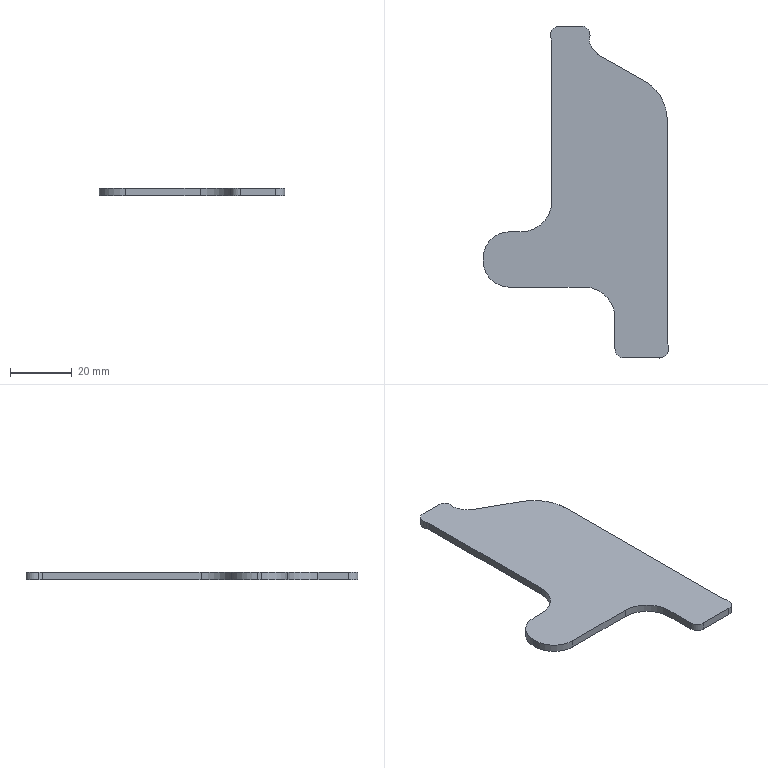Part | STEP file | lll_id346_x_t | 1 solid | 33 faces | box 60.307 x 107.85 x 2.5 mm | volume 8992 mm3 | cylinder 22 | plane 11 | commonest cylinder face diameters 6 x7 17 x2 20 x2 13.156 x1 16.671 x1 21.463 x1
STEP:
#1=CARTESIAN_POINT('',(783.507,50.898,2.5));
#2=VERTEX_POINT('',#1);
#3=CARTESIAN_POINT('',(783.757,49.699,2.5));
#4=VERTEX_POINT('',#3);
#5=CARTESIAN_POINT('',(786.507,50.898,2.5));
#6=DIRECTION('',(0.,0.,1.));
#7=DIRECTION('',(-1.,0.,0.));
#8=AXIS2_PLACEMENT_3D('',#5,#6,#7);
#9=CIRCLE('',#8,3.);
#10=EDGE_CURVE('',#2,#4,#9,.T.);
#11=ORIENTED_EDGE('',*,*,#10,.T.);
#12=CARTESIAN_POINT('',(783.757,49.699,0.));
#13=VERTEX_POINT('',#12);
#14=CARTESIAN_POINT('',(783.757,49.699,0.));
#15=DIRECTION('',(0.,0.,1.));
#16=VECTOR('',#15,1.);
#17=LINE('',#14,#16);
#18=EDGE_CURVE('',#13,#4,#17,.T.);
#19=ORIENTED_EDGE('',*,*,#18,.F.);
#20=CARTESIAN_POINT('',(783.507,50.898,0.));
#21=VERTEX_POINT('',#20);
#22=CARTESIAN_POINT('',(786.507,50.898,0.));
#23=DIRECTION('',(0.,0.,1.));
#24=DIRECTION('',(-1.,0.,0.));
#25=AXIS2_PLACEMENT_3D('',#22,#23,#24);
#26=CIRCLE('',#25,3.);
#27=EDGE_CURVE('',#21,#13,#26,.T.);
#28=ORIENTED_EDGE('',*,*,#27,.F.);
#29=CARTESIAN_POINT('',(783.507,50.898,0.));
#30=DIRECTION('',(0.,0.,1.));
#31=VECTOR('',#30,1.);
#32=LINE('',#29,#31);
#33=EDGE_CURVE('',#21,#2,#32,.T.);
#34=ORIENTED_EDGE('',*,*,#33,.T.);
#35=EDGE_LOOP('',(#11,#19,#28,#34));
#36=FACE_OUTER_BOUND('',#35,.T.);
#37=CARTESIAN_POINT('',(786.507,50.898,0.));
#38=DIRECTION('',(0.,0.,1.));
#39=DIRECTION('',(1.,0.,0.));
#40=AXIS2_PLACEMENT_3D('',#37,#38,#39);
#41=CYLINDRICAL_SURFACE('',#40,3.);
#42=ADVANCED_FACE('',(#36),#41,.F.);
#43=CARTESIAN_POINT('',(781.007,45.5,2.5));
#44=VERTEX_POINT('',#43);
#45=CARTESIAN_POINT('',(781.007,48.5,2.5));
#46=DIRECTION('',(0.,0.,-1.));
#47=DIRECTION('',(-1.,0.,0.));
#48=AXIS2_PLACEMENT_3D('',#45,#46,#47);
#49=CIRCLE('',#48,3.);
#50=EDGE_CURVE('',#4,#44,#49,.T.);
#51=ORIENTED_EDGE('',*,*,#50,.T.);
#52=CARTESIAN_POINT('',(781.007,45.5,0.));
#53=VERTEX_POINT('',#52);
#54=CARTESIAN_POINT('',(781.007,45.5,0.));
#55=DIRECTION('',(0.,0.,1.));
#56=VECTOR('',#55,1.);
#57=LINE('',#54,#56);
#58=EDGE_CURVE('',#53,#44,#57,.T.);
#59=ORIENTED_EDGE('',*,*,#58,.F.);
#60=CARTESIAN_POINT('',(781.007,48.5,0.));
#61=DIRECTION('',(0.,0.,-1.));
#62=DIRECTION('',(-1.,0.,0.));
#63=AXIS2_PLACEMENT_3D('',#60,#61,#62);
#64=CIRCLE('',#63,3.);
#65=EDGE_CURVE('',#13,#53,#64,.T.);
#66=ORIENTED_EDGE('',*,*,#65,.F.);
#67=ORIENTED_EDGE('',*,*,#18,.T.);
#68=EDGE_LOOP('',(#51,#59,#66,#67));
#69=FACE_OUTER_BOUND('',#68,.T.);
#70=CARTESIAN_POINT('',(781.007,48.5,0.));
#71=DIRECTION('',(0.,0.,1.));
#72=DIRECTION('',(1.,0.,0.));
#73=AXIS2_PLACEMENT_3D('',#70,#71,#72);
#74=CYLINDRICAL_SURFACE('',#73,3.);
#75=ADVANCED_FACE('',(#69),#74,.T.);
#76=CARTESIAN_POINT('',(769.5,45.5,2.5));
#77=VERTEX_POINT('',#76);
#78=CARTESIAN_POINT('',(781.007,45.5,2.5));
#79=DIRECTION('',(-1.,0.,0.));
#80=VECTOR('',#79,1.);
#81=LINE('',#78,#80);
#82=EDGE_CURVE('',#44,#77,#81,.T.);
#83=ORIENTED_EDGE('',*,*,#82,.T.);
#84=CARTESIAN_POINT('',(769.5,45.5,0.));
#85=VERTEX_POINT('',#84);
#86=CARTESIAN_POINT('',(769.5,45.5,-2.5));
#87=DIRECTION('',(0.,0.,1.));
#88=VECTOR('',#87,1.);
#89=LINE('',#86,#88);
#90=EDGE_CURVE('',#85,#77,#89,.T.);
#91=ORIENTED_EDGE('',*,*,#90,.F.);
#92=CARTESIAN_POINT('',(781.007,45.5,0.));
#93=DIRECTION('',(-1.,0.,0.));
#94=VECTOR('',#93,1.);
#95=LINE('',#92,#94);
#96=EDGE_CURVE('',#53,#85,#95,.T.);
#97=ORIENTED_EDGE('',*,*,#96,.F.);
#98=ORIENTED_EDGE('',*,*,#58,.T.);
#99=EDGE_LOOP('',(#83,#91,#97,#98));
#100=FACE_OUTER_BOUND('',#99,.T.);
#101=CARTESIAN_POINT('',(781.007,45.5,0.));
#102=DIRECTION('',(0.,1.,0.));
#103=DIRECTION('',(1.,0.,0.));
#104=AXIS2_PLACEMENT_3D('',#101,#102,#103);
#105=PLANE('',#104);
#106=ADVANCED_FACE('',(#100),#105,.F.);
#107=CARTESIAN_POINT('',(766.5,48.5,2.5));
#108=VERTEX_POINT('',#107);
#109=CARTESIAN_POINT('',(766.5,58.5,2.5));
#110=VERTEX_POINT('',#109);
#111=CARTESIAN_POINT('',(766.5,50.898,2.5));
#112=DIRECTION('',(0.,1.,0.));
#113=VECTOR('',#112,1.);
#114=LINE('',#111,#113);
#115=EDGE_CURVE('',#108,#110,#114,.T.);
#116=ORIENTED_EDGE('',*,*,#115,.T.);
#117=CARTESIAN_POINT('',(766.5,58.5,0.));
#118=VERTEX_POINT('',#117);
#119=CARTESIAN_POINT('',(766.5,58.5,0.));
#120=DIRECTION('',(0.,0.,1.));
#121=VECTOR('',#120,1.);
#122=LINE('',#119,#121);
#123=EDGE_CURVE('',#118,#110,#122,.T.);
#124=ORIENTED_EDGE('',*,*,#123,.F.);
#125=CARTESIAN_POINT('',(766.5,48.5,0.));
#126=VERTEX_POINT('',#125);
#127=CARTESIAN_POINT('',(766.5,50.898,0.));
#128=DIRECTION('',(0.,1.,0.));
#129=VECTOR('',#128,1.);
#130=LINE('',#127,#129);
#131=EDGE_CURVE('',#126,#118,#130,.T.);
#132=ORIENTED_EDGE('',*,*,#131,.F.);
#133=CARTESIAN_POINT('',(766.5,48.5,-2.5));
#134=DIRECTION('',(0.,0.,1.));
#135=VECTOR('',#134,1.);
#136=LINE('',#133,#135);
#137=EDGE_CURVE('',#126,#108,#136,.T.);
#138=ORIENTED_EDGE('',*,*,#137,.T.);
#139=EDGE_LOOP('',(#116,#124,#132,#138));
#140=FACE_OUTER_BOUND('',#139,.T.);
#141=CARTESIAN_POINT('',(766.5,50.898,0.));
#142=DIRECTION('',(1.,0.,0.));
#143=DIRECTION('',(0.,0.,-1.));
#144=AXIS2_PLACEMENT_3D('',#141,#142,#143);
#145=PLANE('',#144);
#146=ADVANCED_FACE('',(#140),#145,.F.);
#147=CARTESIAN_POINT('',(756.5,68.5,2.5));
#148=VERTEX_POINT('',#147);
#149=CARTESIAN_POINT('',(756.5,58.5,2.5));
#150=DIRECTION('',(0.,0.,1.));
#151=DIRECTION('',(-1.,0.,0.));
#152=AXIS2_PLACEMENT_3D('',#149,#150,#151);
#153=CIRCLE('',#152,10.);
#154=EDGE_CURVE('',#110,#148,#153,.T.);
#155=ORIENTED_EDGE('',*,*,#154,.T.);
#156=CARTESIAN_POINT('',(756.5,68.5,0.));
#157=VERTEX_POINT('',#156);
#158=CARTESIAN_POINT('',(756.5,68.5,0.));
#159=DIRECTION('',(0.,0.,1.));
#160=VECTOR('',#159,1.);
#161=LINE('',#158,#160);
#162=EDGE_CURVE('',#157,#148,#161,.T.);
#163=ORIENTED_EDGE('',*,*,#162,.F.);
#164=CARTESIAN_POINT('',(756.5,58.5,0.));
#165=DIRECTION('',(0.,0.,1.));
#166=DIRECTION('',(-1.,0.,0.));
#167=AXIS2_PLACEMENT_3D('',#164,#165,#166);
#168=CIRCLE('',#167,10.);
#169=EDGE_CURVE('',#118,#157,#168,.T.);
#170=ORIENTED_EDGE('',*,*,#169,.F.);
#171=ORIENTED_EDGE('',*,*,#123,.T.);
#172=EDGE_LOOP('',(#155,#163,#170,#171));
#173=FACE_OUTER_BOUND('',#172,.T.);
#174=CARTESIAN_POINT('',(756.5,58.5,0.));
#175=DIRECTION('',(0.,0.,1.));
#176=DIRECTION('',(1.,0.,0.));
#177=AXIS2_PLACEMENT_3D('',#174,#175,#176);
#178=CYLINDRICAL_SURFACE('',#177,10.);
#179=ADVANCED_FACE('',(#173),#178,.F.);
#180=CARTESIAN_POINT('',(732.2,68.5,2.5));
#181=VERTEX_POINT('',#180);
#182=CARTESIAN_POINT('',(756.5,68.5,2.5));
#183=DIRECTION('',(-1.,0.,0.));
#184=VECTOR('',#183,1.);
#185=LINE('',#182,#184);
#186=EDGE_CURVE('',#148,#181,#185,.T.);
#187=ORIENTED_EDGE('',*,*,#186,.T.);
#188=CARTESIAN_POINT('',(732.2,68.5,0.));
#189=VERTEX_POINT('',#188);
#190=CARTESIAN_POINT('',(732.2,68.5,0.));
#191=DIRECTION('',(0.,0.,1.));
#192=VECTOR('',#191,1.);
#193=LINE('',#190,#192);
#194=EDGE_CURVE('',#189,#181,#193,.T.);
#195=ORIENTED_EDGE('',*,*,#194,.F.);
#196=CARTESIAN_POINT('',(756.5,68.5,0.));
#197=DIRECTION('',(-1.,0.,0.));
#198=VECTOR('',#197,1.);
#199=LINE('',#196,#198);
#200=EDGE_CURVE('',#157,#189,#199,.T.);
#201=ORIENTED_EDGE('',*,*,#200,.F.);
#202=ORIENTED_EDGE('',*,*,#162,.T.);
#203=EDGE_LOOP('',(#187,#195,#201,#202));
#204=FACE_OUTER_BOUND('',#203,.T.);
#205=CARTESIAN_POINT('',(756.5,68.5,0.));
#206=DIRECTION('',(0.,1.,0.));
#207=DIRECTION('',(0.,0.,1.));
#208=AXIS2_PLACEMENT_3D('',#205,#206,#207);
#209=PLANE('',#208);
#210=ADVANCED_FACE('',(#204),#209,.F.);
#211=CARTESIAN_POINT('',(723.7,77.,2.5));
#212=VERTEX_POINT('',#211);
#213=CARTESIAN_POINT('',(732.2,77.,2.5));
#214=DIRECTION('',(0.,0.,-1.));
#215=DIRECTION('',(-1.,0.,0.));
#216=AXIS2_PLACEMENT_3D('',#213,#214,#215);
#217=CIRCLE('',#216,8.5);
#218=EDGE_CURVE('',#181,#212,#217,.T.);
#219=ORIENTED_EDGE('',*,*,#218,.T.);
#220=CARTESIAN_POINT('',(723.7,77.,0.));
#221=VERTEX_POINT('',#220);
#222=CARTESIAN_POINT('',(723.7,77.,0.));
#223=DIRECTION('',(0.,0.,1.));
#224=VECTOR('',#223,1.);
#225=LINE('',#222,#224);
#226=EDGE_CURVE('',#221,#212,#225,.T.);
#227=ORIENTED_EDGE('',*,*,#226,.F.);
#228=CARTESIAN_POINT('',(732.2,77.,0.));
#229=DIRECTION('',(0.,0.,-1.));
#230=DIRECTION('',(-1.,0.,0.));
#231=AXIS2_PLACEMENT_3D('',#228,#229,#230);
#232=CIRCLE('',#231,8.5);
#233=EDGE_CURVE('',#189,#221,#232,.T.);
#234=ORIENTED_EDGE('',*,*,#233,.F.);
#235=ORIENTED_EDGE('',*,*,#194,.T.);
#236=EDGE_LOOP('',(#219,#227,#234,#235));
#237=FACE_OUTER_BOUND('',#236,.T.);
#238=CARTESIAN_POINT('',(732.2,77.,0.));
#239=DIRECTION('',(0.,0.,1.));
#240=DIRECTION('',(1.,0.,0.));
#241=AXIS2_PLACEMENT_3D('',#238,#239,#240);
#242=CYLINDRICAL_SURFACE('',#241,8.5);
#243=ADVANCED_FACE('',(#237),#242,.T.);
#244=CARTESIAN_POINT('',(723.7,78.,2.5));
#245=VERTEX_POINT('',#244);
#246=CARTESIAN_POINT('',(723.7,77.,2.5));
#247=DIRECTION('',(0.,1.,0.));
#248=VECTOR('',#247,1.);
#249=LINE('',#246,#248);
#250=EDGE_CURVE('',#212,#245,#249,.T.);
#251=ORIENTED_EDGE('',*,*,#250,.T.);
#252=CARTESIAN_POINT('',(723.7,78.,0.));
#253=VERTEX_POINT('',#252);
#254=CARTESIAN_POINT('',(723.7,78.,0.));
#255=DIRECTION('',(0.,0.,1.));
#256=VECTOR('',#255,1.);
#257=LINE('',#254,#256);
#258=EDGE_CURVE('',#253,#245,#257,.T.);
#259=ORIENTED_EDGE('',*,*,#258,.F.);
#260=CARTESIAN_POINT('',(723.7,77.,0.));
#261=DIRECTION('',(0.,1.,0.));
#262=VECTOR('',#261,1.);
#263=LINE('',#260,#262);
#264=EDGE_CURVE('',#221,#253,#263,.T.);
#265=ORIENTED_EDGE('',*,*,#264,.F.);
#266=ORIENTED_EDGE('',*,*,#226,.T.);
#267=EDGE_LOOP('',(#251,#259,#265,#266));
#268=FACE_OUTER_BOUND('',#267,.T.);
#269=CARTESIAN_POINT('',(723.7,77.,0.));
#270=DIRECTION('',(1.,0.,0.));
#271=DIRECTION('',(0.,-1.,0.));
#272=AXIS2_PLACEMENT_3D('',#269,#270,#271);
#273=PLANE('',#272);
#274=ADVANCED_FACE('',(#268),#273,.F.);
#275=CARTESIAN_POINT('',(732.2,86.5,2.5));
#276=VERTEX_POINT('',#275);
#277=CARTESIAN_POINT('',(732.2,78.,2.5));
#278=DIRECTION('',(0.,0.,-1.));
#279=DIRECTION('',(-1.,0.,0.));
#280=AXIS2_PLACEMENT_3D('',#277,#278,#279);
#281=CIRCLE('',#280,8.5);
#282=EDGE_CURVE('',#245,#276,#281,.T.);
#283=ORIENTED_EDGE('',*,*,#282,.T.);
#284=CARTESIAN_POINT('',(732.2,86.5,0.));
#285=VERTEX_POINT('',#284);
#286=CARTESIAN_POINT('',(732.2,86.5,0.));
#287=DIRECTION('',(0.,0.,1.));
#288=VECTOR('',#287,1.);
#289=LINE('',#286,#288);
#290=EDGE_CURVE('',#285,#276,#289,.T.);
#291=ORIENTED_EDGE('',*,*,#290,.F.);
#292=CARTESIAN_POINT('',(732.2,78.,0.));
#293=DIRECTION('',(0.,0.,-1.));
#294=DIRECTION('',(-1.,0.,0.));
#295=AXIS2_PLACEMENT_3D('',#292,#293,#294);
#296=CIRCLE('',#295,8.5);
#297=EDGE_CURVE('',#253,#285,#296,.T.);
#298=ORIENTED_EDGE('',*,*,#297,.F.);
#299=ORIENTED_EDGE('',*,*,#258,.T.);
#300=EDGE_LOOP('',(#283,#291,#298,#299));
#301=FACE_OUTER_BOUND('',#300,.T.);
#302=CARTESIAN_POINT('',(732.2,78.,0.));
#303=DIRECTION('',(0.,0.,1.));
#304=DIRECTION('',(1.,0.,0.));
#305=AXIS2_PLACEMENT_3D('',#302,#303,#304);
#306=CYLINDRICAL_SURFACE('',#305,8.5);
#307=ADVANCED_FACE('',(#301),#306,.T.);
#308=CARTESIAN_POINT('',(736.,86.5,2.5));
#309=VERTEX_POINT('',#308);
#310=CARTESIAN_POINT('',(732.2,86.5,2.5));
#311=DIRECTION('',(1.,0.,0.));
#312=VECTOR('',#311,1.);
#313=LINE('',#310,#312);
#314=EDGE_CURVE('',#276,#309,#313,.T.);
#315=ORIENTED_EDGE('',*,*,#314,.T.);
#316=CARTESIAN_POINT('',(736.,86.5,0.));
#317=VERTEX_POINT('',#316);
#318=CARTESIAN_POINT('',(736.,86.5,0.));
#319=DIRECTION('',(0.,0.,1.));
#320=VECTOR('',#319,1.);
#321=LINE('',#318,#320);
#322=EDGE_CURVE('',#317,#309,#321,.T.);
#323=ORIENTED_EDGE('',*,*,#322,.F.);
#324=CARTESIAN_POINT('',(732.2,86.5,0.));
#325=DIRECTION('',(1.,0.,0.));
#326=VECTOR('',#325,1.);
#327=LINE('',#324,#326);
#328=EDGE_CURVE('',#285,#317,#327,.T.);
#329=ORIENTED_EDGE('',*,*,#328,.F.);
#330=ORIENTED_EDGE('',*,*,#290,.T.);
#331=EDGE_LOOP('',(#315,#323,#329,#330));
#332=FACE_OUTER_BOUND('',#331,.T.);
#333=CARTESIAN_POINT('',(732.2,86.5,0.));
#334=DIRECTION('',(0.,-1.,0.));
#335=DIRECTION('',(0.,0.,-1.));
#336=AXIS2_PLACEMENT_3D('',#333,#334,#335);
#337=PLANE('',#336);
#338=ADVANCED_FACE('',(#332),#337,.F.);
#339=CARTESIAN_POINT('',(746.,96.5,2.5));
#340=VERTEX_POINT('',#339);
#341=CARTESIAN_POINT('',(736.,96.5,2.5));
#342=DIRECTION('',(0.,0.,1.));
#343=DIRECTION('',(-1.,0.,0.));
#344=AXIS2_PLACEMENT_3D('',#341,#342,#343);
#345=CIRCLE('',#344,10.);
#346=EDGE_CURVE('',#309,#340,#345,.T.);
#347=ORIENTED_EDGE('',*,*,#346,.T.);
#348=CARTESIAN_POINT('',(746.,96.5,0.));
#349=VERTEX_POINT('',#348);
#350=CARTESIAN_POINT('',(746.,96.5,0.));
#351=DIRECTION('',(0.,0.,1.));
#352=VECTOR('',#351,1.);
#353=LINE('',#350,#352);
#354=EDGE_CURVE('',#349,#340,#353,.T.);
#355=ORIENTED_EDGE('',*,*,#354,.F.);
#356=CARTESIAN_POINT('',(736.,96.5,0.));
#357=DIRECTION('',(0.,0.,1.));
#358=DIRECTION('',(-1.,0.,0.));
#359=AXIS2_PLACEMENT_3D('',#356,#357,#358);
#360=CIRCLE('',#359,10.);
#361=EDGE_CURVE('',#317,#349,#360,.T.);
#362=ORIENTED_EDGE('',*,*,#361,.F.);
#363=ORIENTED_EDGE('',*,*,#322,.T.);
#364=EDGE_LOOP('',(#347,#355,#362,#363));
#365=FACE_OUTER_BOUND('',#364,.T.);
#366=CARTESIAN_POINT('',(736.,96.5,0.));
#367=DIRECTION('',(0.,0.,1.));
#368=DIRECTION('',(1.,0.,0.));
#369=AXIS2_PLACEMENT_3D('',#366,#367,#368);
#370=CYLINDRICAL_SURFACE('',#369,10.);
#371=ADVANCED_FACE('',(#365),#370,.F.);
#372=CARTESIAN_POINT('',(746.,147.952,2.5));
#373=VERTEX_POINT('',#372);
#374=CARTESIAN_POINT('',(746.,96.5,2.5));
#375=DIRECTION('',(0.,1.,0.));
#376=VECTOR('',#375,1.);
#377=LINE('',#374,#376);
#378=EDGE_CURVE('',#340,#373,#377,.T.);
#379=ORIENTED_EDGE('',*,*,#378,.T.);
#380=CARTESIAN_POINT('',(746.,147.952,0.));
#381=VERTEX_POINT('',#380);
#382=CARTESIAN_POINT('',(746.,147.952,0.));
#383=DIRECTION('',(0.,0.,1.));
#384=VECTOR('',#383,1.);
#385=LINE('',#382,#384);
#386=EDGE_CURVE('',#381,#373,#385,.T.);
#387=ORIENTED_EDGE('',*,*,#386,.F.);
#388=CARTESIAN_POINT('',(746.,96.5,0.));
#389=DIRECTION('',(0.,1.,0.));
#390=VECTOR('',#389,1.);
#391=LINE('',#388,#390);
#392=EDGE_CURVE('',#349,#381,#391,.T.);
#393=ORIENTED_EDGE('',*,*,#392,.F.);
#394=ORIENTED_EDGE('',*,*,#354,.T.);
#395=EDGE_LOOP('',(#379,#387,#393,#394));
#396=FACE_OUTER_BOUND('',#395,.T.);
#397=CARTESIAN_POINT('',(746.,96.5,0.));
#398=DIRECTION('',(1.,0.,0.));
#399=DIRECTION('',(0.,-1.,0.));
#400=AXIS2_PLACEMENT_3D('',#397,#398,#399);
#401=PLANE('',#400);
#402=ADVANCED_FACE('',(#396),#401,.F.);
#403=CARTESIAN_POINT('',(745.75,149.151,2.5));
#404=VERTEX_POINT('',#403);
#405=CARTESIAN_POINT('',(743.,147.952,2.5));
#406=DIRECTION('',(0.,0.,1.));
#407=DIRECTION('',(-1.,0.,0.));
#408=AXIS2_PLACEMENT_3D('',#405,#406,#407);
#409=CIRCLE('',#408,3.);
#410=EDGE_CURVE('',#373,#404,#409,.T.);
#411=ORIENTED_EDGE('',*,*,#410,.T.);
#412=CARTESIAN_POINT('',(745.75,149.151,0.));
#413=VERTEX_POINT('',#412);
#414=CARTESIAN_POINT('',(745.75,149.151,0.));
#415=DIRECTION('',(0.,0.,1.));
#416=VECTOR('',#415,1.);
#417=LINE('',#414,#416);
#418=EDGE_CURVE('',#413,#404,#417,.T.);
#419=ORIENTED_EDGE('',*,*,#418,.F.);
#420=CARTESIAN_POINT('',(743.,147.952,0.));
#421=DIRECTION('',(0.,0.,1.));
#422=DIRECTION('',(-1.,0.,0.));
#423=AXIS2_PLACEMENT_3D('',#420,#421,#422);
#424=CIRCLE('',#423,3.);
#425=EDGE_CURVE('',#381,#413,#424,.T.);
#426=ORIENTED_EDGE('',*,*,#425,.F.);
#427=ORIENTED_EDGE('',*,*,#386,.T.);
#428=EDGE_LOOP('',(#411,#419,#426,#427));
#429=FACE_OUTER_BOUND('',#428,.T.);
#430=CARTESIAN_POINT('',(743.,147.952,0.));
#431=DIRECTION('',(0.,0.,1.));
#432=DIRECTION('',(1.,0.,0.));
#433=AXIS2_PLACEMENT_3D('',#430,#431,#432);
#434=CYLINDRICAL_SURFACE('',#433,3.);
#435=ADVANCED_FACE('',(#429),#434,.F.);
#436=CARTESIAN_POINT('',(748.5,153.35,2.5));
#437=VERTEX_POINT('',#436);
#438=CARTESIAN_POINT('',(748.5,150.35,2.5));
#439=DIRECTION('',(0.,0.,-1.));
#440=DIRECTION('',(-1.,0.,0.));
#441=AXIS2_PLACEMENT_3D('',#438,#439,#440);
#442=CIRCLE('',#441,3.);
#443=EDGE_CURVE('',#404,#437,#442,.T.);
#444=ORIENTED_EDGE('',*,*,#443,.T.);
#445=CARTESIAN_POINT('',(748.5,153.35,0.));
#446=VERTEX_POINT('',#445);
#447=CARTESIAN_POINT('',(748.5,153.35,0.));
#448=DIRECTION('',(0.,0.,1.));
#449=VECTOR('',#448,1.);
#450=LINE('',#447,#449);
#451=EDGE_CURVE('',#446,#437,#450,.T.);
#452=ORIENTED_EDGE('',*,*,#451,.F.);
#453=CARTESIAN_POINT('',(748.5,150.35,0.));
#454=DIRECTION('',(0.,0.,-1.));
#455=DIRECTION('',(-1.,0.,0.));
#456=AXIS2_PLACEMENT_3D('',#453,#454,#455);
#457=CIRCLE('',#456,3.);
#458=EDGE_CURVE('',#413,#446,#457,.T.);
#459=ORIENTED_EDGE('',*,*,#458,.F.);
#460=ORIENTED_EDGE('',*,*,#418,.T.);
#461=EDGE_LOOP('',(#444,#452,#459,#460));
#462=FACE_OUTER_BOUND('',#461,.T.);
#463=CARTESIAN_POINT('',(748.5,150.35,0.));
#464=DIRECTION('',(0.,0.,1.));
#465=DIRECTION('',(1.,0.,0.));
#466=AXIS2_PLACEMENT_3D('',#463,#464,#465);
#467=CYLINDRICAL_SURFACE('',#466,3.);
#468=ADVANCED_FACE('',(#462),#467,.T.);
#469=CARTESIAN_POINT('',(755.404,153.35,2.5));
#470=VERTEX_POINT('',#469);
#471=CARTESIAN_POINT('',(748.5,153.35,2.5));
#472=DIRECTION('',(1.,0.,0.));
#473=VECTOR('',#472,1.);
#474=LINE('',#471,#473);
#475=EDGE_CURVE('',#437,#470,#474,.T.);
#476=ORIENTED_EDGE('',*,*,#475,.T.);
#477=CARTESIAN_POINT('',(755.404,153.35,0.));
#478=VERTEX_POINT('',#477);
#479=CARTESIAN_POINT('',(755.404,153.35,0.));
#480=DIRECTION('',(0.,0.,1.));
#481=VECTOR('',#480,1.);
#482=LINE('',#479,#481);
#483=EDGE_CURVE('',#478,#470,#482,.T.);
#484=ORIENTED_EDGE('',*,*,#483,.F.);
#485=CARTESIAN_POINT('',(748.5,153.35,0.));
#486=DIRECTION('',(1.,0.,0.));
#487=VECTOR('',#486,1.);
#488=LINE('',#485,#487);
#489=EDGE_CURVE('',#446,#478,#488,.T.);
#490=ORIENTED_EDGE('',*,*,#489,.F.);
#491=ORIENTED_EDGE('',*,*,#451,.T.);
#492=EDGE_LOOP('',(#476,#484,#490,#491));
#493=FACE_OUTER_BOUND('',#492,.T.);
#494=CARTESIAN_POINT('',(748.5,153.35,0.));
#495=DIRECTION('',(0.,-1.,0.));
#496=DIRECTION('',(0.,0.,-1.));
#497=AXIS2_PLACEMENT_3D('',#494,#495,#496);
#498=PLANE('',#497);
#499=ADVANCED_FACE('',(#493),#498,.F.);
#500=CARTESIAN_POINT('',(758.292,149.539,2.5));
#501=VERTEX_POINT('',#500);
#502=CARTESIAN_POINT('',(755.404,150.35,2.5));
#503=DIRECTION('',(0.,0.,-1.));
#504=DIRECTION('',(-1.,0.,0.));
#505=AXIS2_PLACEMENT_3D('',#502,#503,#504);
#506=CIRCLE('',#505,3.);
#507=EDGE_CURVE('',#470,#501,#506,.T.);
#508=ORIENTED_EDGE('',*,*,#507,.T.);
#509=CARTESIAN_POINT('',(758.292,149.539,0.));
#510=VERTEX_POINT('',#509);
#511=CARTESIAN_POINT('',(758.292,149.539,0.));
#512=DIRECTION('',(0.,0.,1.));
#513=VECTOR('',#512,1.);
#514=LINE('',#511,#513);
#515=EDGE_CURVE('',#510,#501,#514,.T.);
#516=ORIENTED_EDGE('',*,*,#515,.F.);
#517=CARTESIAN_POINT('',(755.404,150.35,0.));
#518=DIRECTION('',(0.,0.,-1.));
#519=DIRECTION('',(-1.,0.,0.));
#520=AXIS2_PLACEMENT_3D('',#517,#518,#519);
#521=CIRCLE('',#520,3.);
#522=EDGE_CURVE('',#478,#510,#521,.T.);
#523=ORIENTED_EDGE('',*,*,#522,.F.);
#524=ORIENTED_EDGE('',*,*,#483,.T.);
#525=EDGE_LOOP('',(#508,#516,#523,#524));
#526=FACE_OUTER_BOUND('',#525,.T.);
#527=CARTESIAN_POINT('',(755.404,150.35,0.));
#528=DIRECTION('',(0.,0.,1.));
#529=DIRECTION('',(1.,0.,0.));
#530=AXIS2_PLACEMENT_3D('',#527,#528,#529);
#531=CYLINDRICAL_SURFACE('',#530,3.);
#532=ADVANCED_FACE('',(#526),#531,.T.);
#533=CARTESIAN_POINT('',(758.363,147.697,2.5));
#534=VERTEX_POINT('',#533);
#535=CARTESIAN_POINT('',(761.18,148.728,2.5));
#536=DIRECTION('',(0.,0.,1.));
#537=DIRECTION('',(-1.,0.,0.));
#538=AXIS2_PLACEMENT_3D('',#535,#536,#537);
#539=CIRCLE('',#538,3.);
#540=EDGE_CURVE('',#501,#534,#539,.T.);
#541=ORIENTED_EDGE('',*,*,#540,.T.);
#542=CARTESIAN_POINT('',(758.363,147.697,0.));
#543=VERTEX_POINT('',#542);
#544=CARTESIAN_POINT('',(758.363,147.697,0.));
#545=DIRECTION('',(0.,0.,1.));
#546=VECTOR('',#545,1.);
#547=LINE('',#544,#546);
#548=EDGE_CURVE('',#543,#534,#547,.T.);
#549=ORIENTED_EDGE('',*,*,#548,.F.);
#550=CARTESIAN_POINT('',(761.18,148.728,0.));
#551=DIRECTION('',(0.,0.,1.));
#552=DIRECTION('',(-1.,0.,0.));
#553=AXIS2_PLACEMENT_3D('',#550,#551,#552);
#554=CIRCLE('',#553,3.);
#555=EDGE_CURVE('',#510,#543,#554,.T.);
#556=ORIENTED_EDGE('',*,*,#555,.F.);
#557=ORIENTED_EDGE('',*,*,#515,.T.);
#558=EDGE_LOOP('',(#541,#549,#556,#557));
#559=FACE_OUTER_BOUND('',#558,.T.);
#560=CARTESIAN_POINT('',(761.18,148.728,0.));
#561=DIRECTION('',(0.,0.,1.));
#562=DIRECTION('',(1.,0.,0.));
#563=AXIS2_PLACEMENT_3D('',#560,#561,#562);
#564=CYLINDRICAL_SURFACE('',#563,3.);
#565=ADVANCED_FACE('',(#559),#564,.F.);
#566=CARTESIAN_POINT('',(759.773,145.242,2.5));
#567=VERTEX_POINT('',#566);
#568=CARTESIAN_POINT('',(766.191,150.561,2.5));
#569=DIRECTION('',(0.,0.,1.));
#570=DIRECTION('',(-1.,0.,0.));
#571=AXIS2_PLACEMENT_3D('',#568,#569,#570);
#572=CIRCLE('',#571,8.336);
#573=EDGE_CURVE('',#534,#567,#572,.T.);
#574=ORIENTED_EDGE('',*,*,#573,.T.);
#575=CARTESIAN_POINT('',(759.773,145.242,0.));
#576=VERTEX_POINT('',#575);
#577=CARTESIAN_POINT('',(759.773,145.242,0.));
#578=DIRECTION('',(0.,0.,1.));
#579=VECTOR('',#578,1.);
#580=LINE('',#577,#579);
#581=EDGE_CURVE('',#576,#567,#580,.T.);
#582=ORIENTED_EDGE('',*,*,#581,.F.);
#583=CARTESIAN_POINT('',(766.191,150.561,0.));
#584=DIRECTION('',(0.,0.,1.));
#585=DIRECTION('',(-1.,0.,0.));
#586=AXIS2_PLACEMENT_3D('',#583,#584,#585);
#587=CIRCLE('',#586,8.336);
#588=EDGE_CURVE('',#543,#576,#587,.T.);
#589=ORIENTED_EDGE('',*,*,#588,.F.);
#590=ORIENTED_EDGE('',*,*,#548,.T.);
#591=EDGE_LOOP('',(#574,#582,#589,#590));
#592=FACE_OUTER_BOUND('',#591,.T.);
#593=CARTESIAN_POINT('',(766.191,150.561,0.));
#594=DIRECTION('',(0.,0.,1.));
#595=DIRECTION('',(1.,0.,0.));
#596=AXIS2_PLACEMENT_3D('',#593,#594,#595);
#597=CYLINDRICAL_SURFACE('',#596,8.336);
#598=ADVANCED_FACE('',(#592),#597,.F.);
#599=CARTESIAN_POINT('',(760.711,144.326,2.5));
#600=VERTEX_POINT('',#599);
#601=CARTESIAN_POINT('',(764.816,149.465,2.5));
#602=DIRECTION('',(0.,0.,1.));
#603=DIRECTION('',(-1.,0.,0.));
#604=AXIS2_PLACEMENT_3D('',#601,#602,#603);
#605=CIRCLE('',#604,6.578);
#606=EDGE_CURVE('',#567,#600,#605,.T.);
#607=ORIENTED_EDGE('',*,*,#606,.T.);
#608=CARTESIAN_POINT('',(760.711,144.326,0.));
#609=VERTEX_POINT('',#608);
#610=CARTESIAN_POINT('',(760.711,144.326,0.));
#611=DIRECTION('',(0.,0.,1.));
#612=VECTOR('',#611,1.);
#613=LINE('',#610,#612);
#614=EDGE_CURVE('',#609,#600,#613,.T.);
#615=ORIENTED_EDGE('',*,*,#614,.F.);
#616=CARTESIAN_POINT('',(764.816,149.465,0.));
#617=DIRECTION('',(0.,0.,1.));
#618=DIRECTION('',(-1.,0.,0.));
#619=AXIS2_PLACEMENT_3D('',#616,#617,#618);
#620=CIRCLE('',#619,6.578);
#621=EDGE_CURVE('',#576,#609,#620,.T.);
#622=ORIENTED_EDGE('',*,*,#621,.F.);
#623=ORIENTED_EDGE('',*,*,#581,.T.);
#624=EDGE_LOOP('',(#607,#615,#622,#623));
#625=FACE_OUTER_BOUND('',#624,.T.);
#626=CARTESIAN_POINT('',(764.816,149.465,0.));
#627=DIRECTION('',(0.,0.,1.));
#628=DIRECTION('',(1.,0.,0.));
#629=AXIS2_PLACEMENT_3D('',#626,#627,#628);
#630=CYLINDRICAL_SURFACE('',#629,6.578);
#631=ADVANCED_FACE('',(#625),#630,.F.);
#632=CARTESIAN_POINT('',(761.344,143.855,2.5));
#633=VERTEX_POINT('',#632);
#634=CARTESIAN_POINT('',(767.426,152.697,2.5));
#635=DIRECTION('',(0.,0.,1.));
#636=DIRECTION('',(-1.,0.,0.));
#637=AXIS2_PLACEMENT_3D('',#634,#635,#636);
#638=CIRCLE('',#637,10.732);
#639=EDGE_CURVE('',#600,#633,#638,.T.);
#640=ORIENTED_EDGE('',*,*,#639,.T.);
#641=CARTESIAN_POINT('',(761.344,143.855,0.));
#642=VERTEX_POINT('',#641);
#643=CARTESIAN_POINT('',(761.344,143.855,0.));
#644=DIRECTION('',(0.,0.,1.));
#645=VECTOR('',#644,1.);
#646=LINE('',#643,#645);
#647=EDGE_CURVE('',#642,#633,#646,.T.);
#648=ORIENTED_EDGE('',*,*,#647,.F.);
#649=CARTESIAN_POINT('',(767.426,152.697,0.));
#650=DIRECTION('',(0.,0.,1.));
#651=DIRECTION('',(-1.,0.,0.));
#652=AXIS2_PLACEMENT_3D('',#649,#650,#651);
#653=CIRCLE('',#652,10.732);
#654=EDGE_CURVE('',#609,#642,#653,.T.);
#655=ORIENTED_EDGE('',*,*,#654,.F.);
#656=ORIENTED_EDGE('',*,*,#614,.T.);
#657=EDGE_LOOP('',(#640,#648,#655,#656));
#658=FACE_OUTER_BOUND('',#657,.T.);
#659=CARTESIAN_POINT('',(767.426,152.697,0.));
#660=DIRECTION('',(0.,0.,1.));
#661=DIRECTION('',(1.,0.,0.));
#662=AXIS2_PLACEMENT_3D('',#659,#660,#661);
#663=CYLINDRICAL_SURFACE('',#662,10.732);
#664=ADVANCED_FACE('',(#658),#663,.F.);
#665=CARTESIAN_POINT('',(762.002,143.412,2.5));
#666=VERTEX_POINT('',#665);
#667=CARTESIAN_POINT('',(778.7,168.941,2.5));
#668=DIRECTION('',(0.,0.,1.));
#669=DIRECTION('',(-1.,0.,0.));
#670=AXIS2_PLACEMENT_3D('',#667,#668,#669);
#671=CIRCLE('',#670,30.505);
#672=EDGE_CURVE('',#633,#666,#671,.T.);
#673=ORIENTED_EDGE('',*,*,#672,.T.);
#674=CARTESIAN_POINT('',(762.002,143.412,0.));
#675=VERTEX_POINT('',#674);
#676=CARTESIAN_POINT('',(762.002,143.412,0.));
#677=DIRECTION('',(0.,0.,1.));
#678=VECTOR('',#677,1.);
#679=LINE('',#676,#678);
#680=EDGE_CURVE('',#675,#666,#679,.T.);
#681=ORIENTED_EDGE('',*,*,#680,.F.);
#682=CARTESIAN_POINT('',(778.7,168.941,0.));
#683=DIRECTION('',(0.,0.,1.));
#684=DIRECTION('',(-1.,0.,0.));
#685=AXIS2_PLACEMENT_3D('',#682,#683,#684);
#686=CIRCLE('',#685,30.505);
#687=EDGE_CURVE('',#642,#675,#686,.T.);
#688=ORIENTED_EDGE('',*,*,#687,.F.);
#689=ORIENTED_EDGE('',*,*,#647,.T.);
#690=EDGE_LOOP('',(#673,#681,#688,#689));
#691=FACE_OUTER_BOUND('',#690,.T.);
#692=CARTESIAN_POINT('',(778.7,168.941,0.));
#693=DIRECTION('',(0.,0.,1.));
#694=DIRECTION('',(1.,0.,0.));
#695=AXIS2_PLACEMENT_3D('',#692,#693,#694);
#696=CYLINDRICAL_SURFACE('',#695,30.505);
#697=ADVANCED_FACE('',(#691),#696,.F.);
#698=CARTESIAN_POINT('',(775.823,135.647,2.5));
#699=VERTEX_POINT('',#698);
#700=CARTESIAN_POINT('',(762.002,143.412,2.5));
#701=DIRECTION('',(0.8718,-0.4898,0.));
#702=VECTOR('',#701,1.);
#703=LINE('',#700,#702);
#704=EDGE_CURVE('',#666,#699,#703,.T.);
#705=ORIENTED_EDGE('',*,*,#704,.T.);
#706=CARTESIAN_POINT('',(775.823,135.647,0.));
#707=VERTEX_POINT('',#706);
#708=CARTESIAN_POINT('',(775.823,135.647,0.));
#709=DIRECTION('',(0.,0.,1.));
#710=VECTOR('',#709,1.);
#711=LINE('',#708,#710);
#712=EDGE_CURVE('',#707,#699,#711,.T.);
#713=ORIENTED_EDGE('',*,*,#712,.F.);
#714=CARTESIAN_POINT('',(762.002,143.412,0.));
#715=DIRECTION('',(0.8718,-0.4898,0.));
#716=VECTOR('',#715,1.);
#717=LINE('',#714,#716);
#718=EDGE_CURVE('',#675,#707,#717,.T.);
#719=ORIENTED_EDGE('',*,*,#718,.F.);
#720=ORIENTED_EDGE('',*,*,#680,.T.);
#721=EDGE_LOOP('',(#705,#713,#719,#720));
#722=FACE_OUTER_BOUND('',#721,.T.);
#723=CARTESIAN_POINT('',(762.002,143.412,0.));
#724=DIRECTION('',(-0.4898,-0.8718,0.));
#725=DIRECTION('',(-0.8718,0.4898,0.));
#726=AXIS2_PLACEMENT_3D('',#723,#724,#725);
#727=PLANE('',#726);
#728=ADVANCED_FACE('',(#722),#727,.F.);
#729=CARTESIAN_POINT('',(776.661,135.131,2.5));
#730=VERTEX_POINT('',#729);
#731=CARTESIAN_POINT('',(750.344,93.343,2.5));
#732=DIRECTION('',(0.,0.,-1.));
#733=DIRECTION('',(-1.,0.,0.));
#734=AXIS2_PLACEMENT_3D('',#731,#732,#733);
#735=CIRCLE('',#734,49.385);
#736=EDGE_CURVE('',#699,#730,#735,.T.);
#737=ORIENTED_EDGE('',*,*,#736,.T.);
#738=CARTESIAN_POINT('',(776.661,135.131,0.));
#739=VERTEX_POINT('',#738);
#740=CARTESIAN_POINT('',(776.661,135.131,0.));
#741=DIRECTION('',(0.,0.,1.));
#742=VECTOR('',#741,1.);
#743=LINE('',#740,#742);
#744=EDGE_CURVE('',#739,#730,#743,.T.);
#745=ORIENTED_EDGE('',*,*,#744,.F.);
#746=CARTESIAN_POINT('',(750.344,93.343,0.));
#747=DIRECTION('',(0.,0.,-1.));
#748=DIRECTION('',(-1.,0.,0.));
#749=AXIS2_PLACEMENT_3D('',#746,#747,#748);
#750=CIRCLE('',#749,49.385);
#751=EDGE_CURVE('',#707,#739,#750,.T.);
#752=ORIENTED_EDGE('',*,*,#751,.F.);
#753=ORIENTED_EDGE('',*,*,#712,.T.);
#754=EDGE_LOOP('',(#737,#745,#752,#753));
#755=FACE_OUTER_BOUND('',#754,.T.);
#756=CARTESIAN_POINT('',(750.344,93.343,0.));
#757=DIRECTION('',(0.,0.,1.));
#758=DIRECTION('',(1.,0.,0.));
#759=AXIS2_PLACEMENT_3D('',#756,#757,#758);
#760=CYLINDRICAL_SURFACE('',#759,49.385);
#761=ADVANCED_FACE('',(#755),#760,.T.);
#762=CARTESIAN_POINT('',(781.158,130.654,2.5));
#763=VERTEX_POINT('',#762);
#764=CARTESIAN_POINT('',(768.894,122.833,2.5));
#765=DIRECTION('',(0.,0.,-1.));
#766=DIRECTION('',(-1.,0.,0.));
#767=AXIS2_PLACEMENT_3D('',#764,#765,#766);
#768=CIRCLE('',#767,14.545);
#769=EDGE_CURVE('',#730,#763,#768,.T.);
#770=ORIENTED_EDGE('',*,*,#769,.T.);
#771=CARTESIAN_POINT('',(781.158,130.654,0.));
#772=VERTEX_POINT('',#771);
#773=CARTESIAN_POINT('',(781.158,130.654,0.));
#774=DIRECTION('',(0.,0.,1.));
#775=VECTOR('',#774,1.);
#776=LINE('',#773,#775);
#777=EDGE_CURVE('',#772,#763,#776,.T.);
#778=ORIENTED_EDGE('',*,*,#777,.F.);
#779=CARTESIAN_POINT('',(768.894,122.833,0.));
#780=DIRECTION('',(0.,0.,-1.));
#781=DIRECTION('',(-1.,0.,0.));
#782=AXIS2_PLACEMENT_3D('',#779,#780,#781);
#783=CIRCLE('',#782,14.545);
#784=EDGE_CURVE('',#739,#772,#783,.T.);
#785=ORIENTED_EDGE('',*,*,#784,.F.);
#786=ORIENTED_EDGE('',*,*,#744,.T.);
#787=EDGE_LOOP('',(#770,#778,#785,#786));
#788=FACE_OUTER_BOUND('',#787,.T.);
#789=CARTESIAN_POINT('',(768.894,122.833,0.));
#790=DIRECTION('',(0.,0.,1.));
#791=DIRECTION('',(1.,0.,0.));
#792=AXIS2_PLACEMENT_3D('',#789,#790,#791);
#793=CYLINDRICAL_SURFACE('',#792,14.545);
#794=ADVANCED_FACE('',(#788),#793,.T.);
#795=CARTESIAN_POINT('',(782.693,127.563,2.5));
#796=VERTEX_POINT('',#795);
#797=CARTESIAN_POINT('',(768.811,122.594,2.5));
#798=DIRECTION('',(0.,0.,-1.));
#799=DIRECTION('',(-1.,0.,0.));
#800=AXIS2_PLACEMENT_3D('',#797,#798,#799);
#801=CIRCLE('',#800,14.745);
#802=EDGE_CURVE('',#763,#796,#801,.T.);
#803=ORIENTED_EDGE('',*,*,#802,.T.);
#804=CARTESIAN_POINT('',(782.693,127.563,0.));
#805=VERTEX_POINT('',#804);
#806=CARTESIAN_POINT('',(782.693,127.563,0.));
#807=DIRECTION('',(0.,0.,1.));
#808=VECTOR('',#807,1.);
#809=LINE('',#806,#808);
#810=EDGE_CURVE('',#805,#796,#809,.T.);
#811=ORIENTED_EDGE('',*,*,#810,.F.);
#812=CARTESIAN_POINT('',(768.811,122.594,0.));
#813=DIRECTION('',(0.,0.,-1.));
#814=DIRECTION('',(-1.,0.,0.));
#815=AXIS2_PLACEMENT_3D('',#812,#813,#814);
#816=CIRCLE('',#815,14.745);
#817=EDGE_CURVE('',#772,#805,#816,.T.);
#818=ORIENTED_EDGE('',*,*,#817,.F.);
#819=ORIENTED_EDGE('',*,*,#777,.T.);
#820=EDGE_LOOP('',(#803,#811,#818,#819));
#821=FACE_OUTER_BOUND('',#820,.T.);
#822=CARTESIAN_POINT('',(768.811,122.594,0.));
#823=DIRECTION('',(0.,0.,1.));
#824=DIRECTION('',(1.,0.,0.));
#825=AXIS2_PLACEMENT_3D('',#822,#823,#824);
#826=CYLINDRICAL_SURFACE('',#825,14.745);
#827=ADVANCED_FACE('',(#821),#826,.T.);
#828=CARTESIAN_POINT('',(783.185,125.664,2.5));
#829=VERTEX_POINT('',#828);
#830=CARTESIAN_POINT('',(771.686,123.7,2.5));
#831=DIRECTION('',(0.,0.,-1.));
#832=DIRECTION('',(-1.,0.,0.));
#833=AXIS2_PLACEMENT_3D('',#830,#831,#832);
#834=CIRCLE('',#833,11.666);
#835=EDGE_CURVE('',#796,#829,#834,.T.);
#836=ORIENTED_EDGE('',*,*,#835,.T.);
#837=CARTESIAN_POINT('',(783.185,125.664,0.));
#838=VERTEX_POINT('',#837);
#839=CARTESIAN_POINT('',(783.185,125.664,0.));
#840=DIRECTION('',(0.,0.,1.));
#841=VECTOR('',#840,1.);
#842=LINE('',#839,#841);
#843=EDGE_CURVE('',#838,#829,#842,.T.);
#844=ORIENTED_EDGE('',*,*,#843,.F.);
#845=CARTESIAN_POINT('',(771.686,123.7,0.));
#846=DIRECTION('',(0.,0.,-1.));
#847=DIRECTION('',(-1.,0.,0.));
#848=AXIS2_PLACEMENT_3D('',#845,#846,#847);
#849=CIRCLE('',#848,11.666);
#850=EDGE_CURVE('',#805,#838,#849,.T.);
#851=ORIENTED_EDGE('',*,*,#850,.F.);
#852=ORIENTED_EDGE('',*,*,#810,.T.);
#853=EDGE_LOOP('',(#836,#844,#851,#852));
#854=FACE_OUTER_BOUND('',#853,.T.);
#855=CARTESIAN_POINT('',(771.686,123.7,0.));
#856=DIRECTION('',(0.,0.,1.));
#857=DIRECTION('',(1.,0.,0.));
#858=AXIS2_PLACEMENT_3D('',#855,#856,#857);
#859=CYLINDRICAL_SURFACE('',#858,11.666);
#860=ADVANCED_FACE('',(#854),#859,.T.);
#861=CARTESIAN_POINT('',(783.326,124.692,2.5));
#862=VERTEX_POINT('',#861);
#863=CARTESIAN_POINT('',(765.809,122.646,2.5));
#864=DIRECTION('',(0.,0.,-1.));
#865=DIRECTION('',(-1.,0.,0.));
#866=AXIS2_PLACEMENT_3D('',#863,#864,#865);
#867=CIRCLE('',#866,17.636);
#868=EDGE_CURVE('',#829,#862,#867,.T.);
#869=ORIENTED_EDGE('',*,*,#868,.T.);
#870=CARTESIAN_POINT('',(783.326,124.692,0.));
#871=VERTEX_POINT('',#870);
#872=CARTESIAN_POINT('',(783.326,124.692,0.));
#873=DIRECTION('',(0.,0.,1.));
#874=VECTOR('',#873,1.);
#875=LINE('',#872,#874);
#876=EDGE_CURVE('',#871,#862,#875,.T.);
#877=ORIENTED_EDGE('',*,*,#876,.F.);
#878=CARTESIAN_POINT('',(765.809,122.646,0.));
#879=DIRECTION('',(0.,0.,-1.));
#880=DIRECTION('',(-1.,0.,0.));
#881=AXIS2_PLACEMENT_3D('',#878,#879,#880);
#882=CIRCLE('',#881,17.636);
#883=EDGE_CURVE('',#838,#871,#882,.T.);
#884=ORIENTED_EDGE('',*,*,#883,.F.);
#885=ORIENTED_EDGE('',*,*,#843,.T.);
#886=EDGE_LOOP('',(#869,#877,#884,#885));
#887=FACE_OUTER_BOUND('',#886,.T.);
#888=CARTESIAN_POINT('',(765.809,122.646,0.));
#889=DIRECTION('',(0.,0.,1.));
#890=DIRECTION('',(1.,0.,0.));
#891=AXIS2_PLACEMENT_3D('',#888,#889,#890);
#892=CYLINDRICAL_SURFACE('',#891,17.636);
#893=ADVANCED_FACE('',(#887),#892,.T.);
#894=CARTESIAN_POINT('',(783.424,123.71,2.5));
#895=VERTEX_POINT('',#894);
#896=CARTESIAN_POINT('',(753.776,121.24,2.5));
#897=DIRECTION('',(0.,0.,-1.));
#898=DIRECTION('',(-1.,0.,0.));
#899=AXIS2_PLACEMENT_3D('',#896,#897,#898);
#900=CIRCLE('',#899,29.75);
#901=EDGE_CURVE('',#862,#895,#900,.T.);
#902=ORIENTED_EDGE('',*,*,#901,.T.);
#903=CARTESIAN_POINT('',(783.424,123.71,0.));
#904=VERTEX_POINT('',#903);
#905=CARTESIAN_POINT('',(783.424,123.71,0.));
#906=DIRECTION('',(0.,0.,1.));
#907=VECTOR('',#906,1.);
#908=LINE('',#905,#907);
#909=EDGE_CURVE('',#904,#895,#908,.T.);
#910=ORIENTED_EDGE('',*,*,#909,.F.);
#911=CARTESIAN_POINT('',(753.776,121.24,0.));
#912=DIRECTION('',(0.,0.,-1.));
#913=DIRECTION('',(-1.,0.,0.));
#914=AXIS2_PLACEMENT_3D('',#911,#912,#913);
#915=CIRCLE('',#914,29.75);
#916=EDGE_CURVE('',#871,#904,#915,.T.);
#917=ORIENTED_EDGE('',*,*,#916,.F.);
#918=ORIENTED_EDGE('',*,*,#876,.T.);
#919=EDGE_LOOP('',(#902,#910,#917,#918));
#920=FACE_OUTER_BOUND('',#919,.T.);
#921=CARTESIAN_POINT('',(753.776,121.24,0.));
#922=DIRECTION('',(0.,0.,1.));
#923=DIRECTION('',(1.,0.,0.));
#924=AXIS2_PLACEMENT_3D('',#921,#922,#923);
#925=CYLINDRICAL_SURFACE('',#924,29.75);
#926=ADVANCED_FACE('',(#920),#925,.T.);
#927=CARTESIAN_POINT('',(783.501,122.723,2.5));
#928=VERTEX_POINT('',#927);
#929=CARTESIAN_POINT('',(729.763,119.039,2.5));
#930=DIRECTION('',(0.,0.,-1.));
#931=DIRECTION('',(-1.,0.,0.));
#932=AXIS2_PLACEMENT_3D('',#929,#930,#931);
#933=CIRCLE('',#932,53.864);
#934=EDGE_CURVE('',#895,#928,#933,.T.);
#935=ORIENTED_EDGE('',*,*,#934,.T.);
#936=CARTESIAN_POINT('',(783.501,122.723,0.));
#937=VERTEX_POINT('',#936);
#938=CARTESIAN_POINT('',(783.501,122.723,0.));
#939=DIRECTION('',(0.,0.,1.));
#940=VECTOR('',#939,1.);
#941=LINE('',#938,#940);
#942=EDGE_CURVE('',#937,#928,#941,.T.);
#943=ORIENTED_EDGE('',*,*,#942,.F.);
#944=CARTESIAN_POINT('',(729.763,119.039,0.));
#945=DIRECTION('',(0.,0.,-1.));
#946=DIRECTION('',(-1.,0.,0.));
#947=AXIS2_PLACEMENT_3D('',#944,#945,#946);
#948=CIRCLE('',#947,53.864);
#949=EDGE_CURVE('',#904,#937,#948,.T.);
#950=ORIENTED_EDGE('',*,*,#949,.F.);
#951=ORIENTED_EDGE('',*,*,#909,.T.);
#952=EDGE_LOOP('',(#935,#943,#950,#951));
#953=FACE_OUTER_BOUND('',#952,.T.);
#954=CARTESIAN_POINT('',(729.763,119.039,0.));
#955=DIRECTION('',(0.,0.,1.));
#956=DIRECTION('',(1.,0.,0.));
#957=AXIS2_PLACEMENT_3D('',#954,#955,#956);
#958=CYLINDRICAL_SURFACE('',#957,53.864);
#959=ADVANCED_FACE('',(#953),#958,.T.);
#960=CARTESIAN_POINT('',(783.501,122.723,2.5));
#961=DIRECTION('',(0.00008308,-1.,0.));
#962=VECTOR('',#961,1.);
#963=LINE('',#960,#962);
#964=EDGE_CURVE('',#928,#2,#963,.T.);
#965=ORIENTED_EDGE('',*,*,#964,.T.);
#966=ORIENTED_EDGE('',*,*,#33,.F.);
#967=CARTESIAN_POINT('',(783.501,122.723,0.));
#968=DIRECTION('',(0.00008308,-1.,0.));
#969=VECTOR('',#968,1.);
#970=LINE('',#967,#969);
#971=EDGE_CURVE('',#937,#21,#970,.T.);
#972=ORIENTED_EDGE('',*,*,#971,.F.);
#973=ORIENTED_EDGE('',*,*,#942,.T.);
#974=EDGE_LOOP('',(#965,#966,#972,#973));
#975=FACE_OUTER_BOUND('',#974,.T.);
#976=CARTESIAN_POINT('',(783.501,122.723,0.));
#977=DIRECTION('',(-1.,-0.00008308,0.));
#978=DIRECTION('',(-0.00008308,1.,0.));
#979=AXIS2_PLACEMENT_3D('',#976,#977,#978);
#980=PLANE('',#979);
#981=ADVANCED_FACE('',(#975),#980,.F.);
#982=ORIENTED_EDGE('',*,*,#96,.T.);
#983=CARTESIAN_POINT('',(769.5,48.5,0.));
#984=DIRECTION('',(0.,0.,1.));
#985=DIRECTION('',(1.,0.,0.));
#986=AXIS2_PLACEMENT_3D('',#983,#984,#985);
#987=CIRCLE('',#986,3.);
#988=EDGE_CURVE('',#126,#85,#987,.T.);
#989=ORIENTED_EDGE('',*,*,#988,.F.);
#990=ORIENTED_EDGE('',*,*,#131,.T.);
#991=ORIENTED_EDGE('',*,*,#169,.T.);
#992=ORIENTED_EDGE('',*,*,#200,.T.);
#993=ORIENTED_EDGE('',*,*,#233,.T.);
#994=ORIENTED_EDGE('',*,*,#264,.T.);
#995=ORIENTED_EDGE('',*,*,#297,.T.);
#996=ORIENTED_EDGE('',*,*,#328,.T.);
#997=ORIENTED_EDGE('',*,*,#361,.T.);
#998=ORIENTED_EDGE('',*,*,#392,.T.);
#999=ORIENTED_EDGE('',*,*,#425,.T.);
#1000=ORIENTED_EDGE('',*,*,#458,.T.);
#1001=ORIENTED_EDGE('',*,*,#489,.T.);
#1002=ORIENTED_EDGE('',*,*,#522,.T.);
#1003=ORIENTED_EDGE('',*,*,#555,.T.);
#1004=ORIENTED_EDGE('',*,*,#588,.T.);
#1005=ORIENTED_EDGE('',*,*,#621,.T.);
#1006=ORIENTED_EDGE('',*,*,#654,.T.);
#1007=ORIENTED_EDGE('',*,*,#687,.T.);
#1008=ORIENTED_EDGE('',*,*,#718,.T.);
#1009=ORIENTED_EDGE('',*,*,#751,.T.);
#1010=ORIENTED_EDGE('',*,*,#784,.T.);
#1011=ORIENTED_EDGE('',*,*,#817,.T.);
#1012=ORIENTED_EDGE('',*,*,#850,.T.);
#1013=ORIENTED_EDGE('',*,*,#883,.T.);
#1014=ORIENTED_EDGE('',*,*,#916,.T.);
#1015=ORIENTED_EDGE('',*,*,#949,.T.);
#1016=ORIENTED_EDGE('',*,*,#971,.T.);
#1017=ORIENTED_EDGE('',*,*,#27,.T.);
#1018=ORIENTED_EDGE('',*,*,#65,.T.);
#1019=EDGE_LOOP('',(#982,#989,#990,#991,#992,#993,#994,#995,#996,#997,#998,#999,#1000,#1001,#1002,#1003,#1004,#1005,#1006,#1007,#1008,#1009,#1010,#1011,#1012,#1013,#1014,#1015,#1016,#1017,#1018));
#1020=FACE_OUTER_BOUND('',#1019,.T.);
#1021=CARTESIAN_POINT('',(786.507,50.898,0.));
#1022=DIRECTION('',(0.,0.,1.));
#1023=DIRECTION('',(1.,0.,0.));
#1024=AXIS2_PLACEMENT_3D('',#1021,#1022,#1023);
#1025=PLANE('',#1024);
#1026=ADVANCED_FACE('',(#1020),#1025,.F.);
#1027=CARTESIAN_POINT('',(769.5,48.5,2.5));
#1028=DIRECTION('',(0.,0.,-1.));
#1029=DIRECTION('',(1.,0.,0.));
#1030=AXIS2_PLACEMENT_3D('',#1027,#1028,#1029);
#1031=CIRCLE('',#1030,3.);
#1032=EDGE_CURVE('',#77,#108,#1031,.T.);
#1033=ORIENTED_EDGE('',*,*,#1032,.F.);
#1034=ORIENTED_EDGE('',*,*,#82,.F.);
#1035=ORIENTED_EDGE('',*,*,#50,.F.);
#1036=ORIENTED_EDGE('',*,*,#10,.F.);
#1037=ORIENTED_EDGE('',*,*,#964,.F.);
#1038=ORIENTED_EDGE('',*,*,#934,.F.);
#1039=ORIENTED_EDGE('',*,*,#901,.F.);
#1040=ORIENTED_EDGE('',*,*,#868,.F.);
#1041=ORIENTED_EDGE('',*,*,#835,.F.);
#1042=ORIENTED_EDGE('',*,*,#802,.F.);
#1043=ORIENTED_EDGE('',*,*,#769,.F.);
#1044=ORIENTED_EDGE('',*,*,#736,.F.);
#1045=ORIENTED_EDGE('',*,*,#704,.F.);
#1046=ORIENTED_EDGE('',*,*,#672,.F.);
#1047=ORIENTED_EDGE('',*,*,#639,.F.);
#1048=ORIENTED_EDGE('',*,*,#606,.F.);
#1049=ORIENTED_EDGE('',*,*,#573,.F.);
#1050=ORIENTED_EDGE('',*,*,#540,.F.);
#1051=ORIENTED_EDGE('',*,*,#507,.F.);
#1052=ORIENTED_EDGE('',*,*,#475,.F.);
#1053=ORIENTED_EDGE('',*,*,#443,.F.);
#1054=ORIENTED_EDGE('',*,*,#410,.F.);
#1055=ORIENTED_EDGE('',*,*,#378,.F.);
#1056=ORIENTED_EDGE('',*,*,#346,.F.);
#1057=ORIENTED_EDGE('',*,*,#314,.F.);
#1058=ORIENTED_EDGE('',*,*,#282,.F.);
#1059=ORIENTED_EDGE('',*,*,#250,.F.);
#1060=ORIENTED_EDGE('',*,*,#218,.F.);
#1061=ORIENTED_EDGE('',*,*,#186,.F.);
#1062=ORIENTED_EDGE('',*,*,#154,.F.);
#1063=ORIENTED_EDGE('',*,*,#115,.F.);
#1064=EDGE_LOOP('',(#1033,#1034,#1035,#1036,#1037,#1038,#1039,#1040,#1041,#1042,#1043,#1044,#1045,#1046,#1047,#1048,#1049,#1050,#1051,#1052,#1053,#1054,#1055,#1056,#1057,#1058,#1059,#1060,#1061,#1062,#1063));
#1065=FACE_OUTER_BOUND('',#1064,.T.);
#1066=CARTESIAN_POINT('',(786.507,50.898,2.5));
#1067=DIRECTION('',(0.,0.,1.));
#1068=DIRECTION('',(1.,0.,0.));
#1069=AXIS2_PLACEMENT_3D('',#1066,#1067,#1068);
#1070=PLANE('',#1069);
#1071=ADVANCED_FACE('',(#1065),#1070,.T.);
#1072=ORIENTED_EDGE('',*,*,#90,.T.);
#1073=ORIENTED_EDGE('',*,*,#1032,.T.);
#1074=ORIENTED_EDGE('',*,*,#137,.F.);
#1075=ORIENTED_EDGE('',*,*,#988,.T.);
#1076=EDGE_LOOP('',(#1072,#1073,#1074,#1075));
#1077=FACE_OUTER_BOUND('',#1076,.T.);
#1078=CARTESIAN_POINT('',(769.5,48.5,-2.5));
#1079=DIRECTION('',(0.,0.,1.));
#1080=DIRECTION('',(1.,0.,0.));
#1081=AXIS2_PLACEMENT_3D('',#1078,#1079,#1080);
#1082=CYLINDRICAL_SURFACE('',#1081,3.);
#1083=ADVANCED_FACE('',(#1077),#1082,.T.);
#1084=CLOSED_SHELL('',(#42,#75,#106,#146,#179,#210,#243,#274,#307,#338,#371,#402,#435,#468,#499,#532,#565,#598,#631,#664,#697,#728,#761,#794,#827,#860,#893,#926,#959,#981,#1026,#1071,#1083));
#1085=MANIFOLD_SOLID_BREP('',#1084);
#1086=(LENGTH_UNIT()NAMED_UNIT(*)SI_UNIT(.MILLI.,.METRE.));
#1087=UNCERTAINTY_MEASURE_WITH_UNIT(LENGTH_MEASURE(0.00002),#1086,'','');
#1088=(NAMED_UNIT(*)PLANE_ANGLE_UNIT()SI_UNIT($,.RADIAN.));
#1089=PLANE_ANGLE_MEASURE_WITH_UNIT(PLANE_ANGLE_MEASURE(0.01745),#1088);
#1090=DIMENSIONAL_EXPONENTS(0.,0.,0.,0.,0.,0.,0.);
#1091=(CONVERSION_BASED_UNIT('DEGREE',#1089)NAMED_UNIT(#1090)PLANE_ANGLE_UNIT());
#1092=(NAMED_UNIT(*)SI_UNIT($,.STERADIAN.)SOLID_ANGLE_UNIT());
#1093=(GEOMETRIC_REPRESENTATION_CONTEXT(3)GLOBAL_UNCERTAINTY_ASSIGNED_CONTEXT((#1087))GLOBAL_UNIT_ASSIGNED_CONTEXT((#1086,#1091,#1092))REPRESENTATION_CONTEXT('',''));
#1094=ADVANCED_BREP_SHAPE_REPRESENTATION('',(#1085),#1093);